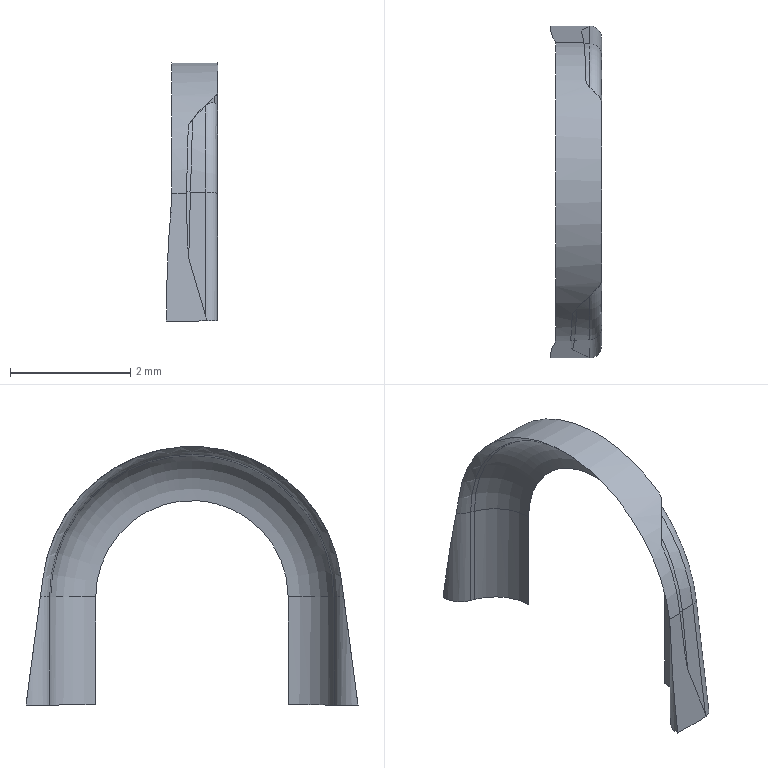Part | STEP file | Basler ace 2 USB3-1-1-1_2 | 1 solid | 37 faces | box 0.85 x 5.522 x 4.3 mm | volume 2.556 mm3 | plane 16 | cylinder 11 | torus 6 | cone 3 | spline 1 | commonest cylinder face diameters 0.4 x4 0.8 x2 1.6 x2 0.3 x1 0.6 x1 5 x1
STEP:
#1=CARTESIAN_POINT('',(-13.565,6.449,-26.303));
#2=VERTEX_POINT('',#1);
#3=CARTESIAN_POINT('',(-13.345,6.67,-26.068));
#4=VERTEX_POINT('',#3);
#5=CARTESIAN_POINT('',(-11.678,8.336,-27.85));
#6=DIRECTION('',(-0.7071,0.7071,0.));
#7=DIRECTION('',(0.7071,0.7071,0.));
#8=AXIS2_PLACEMENT_3D('',#5,#6,#7);
#9=ELLIPSE('',#8,3.451,2.44);
#10=EDGE_CURVE('',#2,#4,#9,.T.);
#11=ORIENTED_EDGE('',*,*,#10,.F.);
#12=CARTESIAN_POINT('',(-13.6,5.933,-27.503));
#13=VERTEX_POINT('',#12);
#14=CARTESIAN_POINT('',(-13.604,7.833,-27.608));
#15=DIRECTION('',(-0.9996,0.000003627,0.02933));
#16=DIRECTION('',(0.02696,0.3938,0.9188));
#17=AXIS2_PLACEMENT_3D('',#14,#15,#16);
#18=ELLIPSE('',#17,2.174,1.873);
#19=EDGE_CURVE('',#13,#2,#18,.T.);
#20=ORIENTED_EDGE('',*,*,#19,.F.);
#21=CARTESIAN_POINT('',(-13.345,5.94,-27.504));
#22=VERTEX_POINT('',#21);
#23=CARTESIAN_POINT('',(-13.345,5.94,-27.504));
#24=DIRECTION('',(-0.9997,-0.02592,0.003643));
#25=VECTOR('',#24,10.);
#26=LINE('',#23,#25);
#27=EDGE_CURVE('',#22,#13,#26,.T.);
#28=ORIENTED_EDGE('',*,*,#27,.F.);
#29=CARTESIAN_POINT('',(-13.345,8.4,-27.85));
#30=DIRECTION('',(1.,0.,0.));
#31=DIRECTION('',(0.,-0.9903,0.1392));
#32=AXIS2_PLACEMENT_3D('',#29,#30,#31);
#33=CIRCLE('',#32,2.484);
#34=EDGE_CURVE('',#4,#22,#33,.T.);
#35=ORIENTED_EDGE('',*,*,#34,.F.);
#36=EDGE_LOOP('',(#11,#20,#28,#35));
#37=FACE_OUTER_BOUND('',#36,.T.);
#38=CARTESIAN_POINT('',(-13.95,8.4,-27.85));
#39=DIRECTION('',(-1.,0.,0.));
#40=DIRECTION('',(0.,-0.9903,-0.1392));
#41=AXIS2_PLACEMENT_3D('',#38,#39,#40);
#42=CONICAL_SURFACE('',#41,2.5,0.02618);
#43=ADVANCED_FACE('',(#37),#42,.T.);
#44=CARTESIAN_POINT('',(-14.,5.639,-29.65));
#45=VERTEX_POINT('',#44);
#46=CARTESIAN_POINT('',(-14.,5.65,-29.65));
#47=VERTEX_POINT('',#46);
#48=CARTESIAN_POINT('',(-14.,5.65,-29.65));
#49=DIRECTION('',(0.,-1.,0.));
#50=VECTOR('',#49,0.011);
#51=LINE('',#48,#50);
#52=EDGE_CURVE('',#45,#47,#51,.F.);
#53=ORIENTED_EDGE('',*,*,#52,.F.);
#54=CARTESIAN_POINT('',(-14.,5.65,-29.567));
#55=VERTEX_POINT('',#54);
#56=CARTESIAN_POINT('',(-14.,5.65,-29.567));
#57=DIRECTION('',(0.,-0.1316,-0.9913));
#58=VECTOR('',#57,0.08356);
#59=LINE('',#56,#58);
#60=EDGE_CURVE('',#55,#45,#59,.T.);
#61=ORIENTED_EDGE('',*,*,#60,.F.);
#62=CARTESIAN_POINT('',(-14.,5.65,-29.65));
#63=DIRECTION('',(0.,0.,1.));
#64=VECTOR('',#63,10.);
#65=LINE('',#62,#64);
#66=EDGE_CURVE('',#47,#55,#65,.T.);
#67=ORIENTED_EDGE('',*,*,#66,.F.);
#68=EDGE_LOOP('',(#53,#61,#67));
#69=FACE_OUTER_BOUND('',#68,.T.);
#70=CARTESIAN_POINT('',(-14.,4.591,-15.027));
#71=DIRECTION('',(1.,0.,0.));
#72=DIRECTION('',(0.,0.,-1.));
#73=AXIS2_PLACEMENT_3D('',#70,#71,#72);
#74=PLANE('',#73);
#75=ADVANCED_FACE('',(#69),#74,.F.);
#76=CARTESIAN_POINT('',(-13.5,5.639,-29.65));
#77=VERTEX_POINT('',#76);
#78=CARTESIAN_POINT('',(-13.5,5.639,-29.65));
#79=DIRECTION('',(-1.,0.,0.));
#80=VECTOR('',#79,0.5);
#81=LINE('',#78,#80);
#82=EDGE_CURVE('',#45,#77,#81,.F.);
#83=ORIENTED_EDGE('',*,*,#82,.F.);
#84=ORIENTED_EDGE('',*,*,#52,.T.);
#85=CARTESIAN_POINT('',(-13.739,6.025,-29.65));
#86=VERTEX_POINT('',#85);
#87=CARTESIAN_POINT('',(-13.6,5.65,-29.65));
#88=DIRECTION('',(0.,0.,-1.));
#89=DIRECTION('',(0.,1.,0.));
#90=AXIS2_PLACEMENT_3D('',#87,#88,#89);
#91=CIRCLE('',#90,0.4);
#92=EDGE_CURVE('',#86,#47,#91,.F.);
#93=ORIENTED_EDGE('',*,*,#92,.F.);
#94=CARTESIAN_POINT('',(-13.672,6.05,-29.65));
#95=VERTEX_POINT('',#94);
#96=CARTESIAN_POINT('',(-13.739,6.025,-29.65));
#97=DIRECTION('',(0.9379,0.3469,0.));
#98=VECTOR('',#97,0.07071);
#99=LINE('',#96,#98);
#100=EDGE_CURVE('',#86,#95,#99,.T.);
#101=ORIENTED_EDGE('',*,*,#100,.T.);
#102=CARTESIAN_POINT('',(-13.5,6.139,-29.65));
#103=VERTEX_POINT('',#102);
#104=CARTESIAN_POINT('',(-13.95,6.8,-29.65));
#105=DIRECTION('',(0.,0.,-1.));
#106=DIRECTION('',(0.,1.,0.));
#107=AXIS2_PLACEMENT_3D('',#104,#105,#106);
#108=CIRCLE('',#107,0.8);
#109=EDGE_CURVE('',#95,#103,#108,.F.);
#110=ORIENTED_EDGE('',*,*,#109,.T.);
#111=CARTESIAN_POINT('',(-13.5,5.639,-29.65));
#112=DIRECTION('',(0.,1.,0.));
#113=VECTOR('',#112,10.);
#114=LINE('',#111,#113);
#115=EDGE_CURVE('',#77,#103,#114,.T.);
#116=ORIENTED_EDGE('',*,*,#115,.F.);
#117=EDGE_LOOP('',(#83,#84,#93,#101,#110,#116));
#118=FACE_OUTER_BOUND('',#117,.T.);
#119=CARTESIAN_POINT('',(-14.2,5.639,-29.65));
#120=DIRECTION('',(0.,0.,-1.));
#121=DIRECTION('',(-1.,0.,0.));
#122=AXIS2_PLACEMENT_3D('',#119,#120,#121);
#123=PLANE('',#122);
#124=ADVANCED_FACE('',(#118),#123,.T.);
#125=CARTESIAN_POINT('',(-13.629,5.777,-28.608));
#126=VERTEX_POINT('',#125);
#127=CARTESIAN_POINT('',(-13.6,5.933,-27.503));
#128=DIRECTION('',(-0.02592,-0.1398,-0.9898));
#129=VECTOR('',#128,10.);
#130=LINE('',#127,#129);
#131=EDGE_CURVE('',#13,#126,#130,.T.);
#132=ORIENTED_EDGE('',*,*,#131,.T.);
#133=CARTESIAN_POINT('',(-13.345,5.648,-29.58));
#134=VERTEX_POINT('',#133);
#135=CARTESIAN_POINT('',(-13.345,5.648,-29.58));
#136=DIRECTION('',(-0.2785,0.1264,0.9521));
#137=VECTOR('',#136,10.);
#138=LINE('',#135,#137);
#139=EDGE_CURVE('',#134,#126,#138,.T.);
#140=ORIENTED_EDGE('',*,*,#139,.F.);
#141=CARTESIAN_POINT('',(-13.345,5.94,-27.504));
#142=DIRECTION('',(0.,-0.1392,-0.9903));
#143=VECTOR('',#142,10.);
#144=LINE('',#141,#143);
#145=EDGE_CURVE('',#22,#134,#144,.T.);
#146=ORIENTED_EDGE('',*,*,#145,.F.);
#147=ORIENTED_EDGE('',*,*,#27,.T.);
#148=EDGE_LOOP('',(#132,#140,#146,#147));
#149=FACE_OUTER_BOUND('',#148,.T.);
#150=CARTESIAN_POINT('',(-13.95,5.621,-29.662));
#151=DIRECTION('',(0.02618,-0.9899,0.1391));
#152=DIRECTION('',(0.,-0.1392,-0.9903));
#153=AXIS2_PLACEMENT_3D('',#150,#151,#152);
#154=PLANE('',#153);
#155=ADVANCED_FACE('',(#149),#154,.T.);
#156=CARTESIAN_POINT('',(-13.667,5.925,-27.5));
#157=VERTEX_POINT('',#156);
#158=CARTESIAN_POINT('',(-13.593,5.636,-27.462));
#159=DIRECTION('',(-0.02592,-0.1398,-0.9898));
#160=DIRECTION('',(-0.02631,0.9899,-0.1391));
#161=AXIS2_PLACEMENT_3D('',#158,#159,#160);
#162=CIRCLE('',#161,0.3004);
#163=EDGE_CURVE('',#157,#13,#162,.T.);
#164=ORIENTED_EDGE('',*,*,#163,.F.);
#165=CARTESIAN_POINT('',(-13.667,5.922,-27.521));
#166=VERTEX_POINT('',#165);
#167=CARTESIAN_POINT('',(-13.652,5.927,-27.513));
#168=DIRECTION('',(-0.2453,0.9608,-0.1293));
#169=DIRECTION('',(0.00731,0.1352,0.9908));
#170=AXIS2_PLACEMENT_3D('',#167,#168,#169);
#171=ELLIPSE('',#170,0.09616,0.01504);
#172=EDGE_CURVE('',#166,#157,#171,.T.);
#173=ORIENTED_EDGE('',*,*,#172,.F.);
#174=CARTESIAN_POINT('',(-13.629,5.777,-28.608));
#175=CARTESIAN_POINT('',(-13.66,5.791,-28.503));
#176=CARTESIAN_POINT('',(-13.667,5.922,-27.521));
#177=(BOUNDED_CURVE()B_SPLINE_CURVE(2,(#174,#175,#176),.UNSPECIFIED.,.F.,.F.)B_SPLINE_CURVE_WITH_KNOTS((3,3),(0.2462,0.3879),.UNSPECIFIED.)CURVE()GEOMETRIC_REPRESENTATION_ITEM()RATIONAL_B_SPLINE_CURVE((0.9685,0.9699,0.9834))REPRESENTATION_ITEM(''));
#178=EDGE_CURVE('',#126,#166,#177,.T.);
#179=ORIENTED_EDGE('',*,*,#178,.F.);
#180=ORIENTED_EDGE('',*,*,#131,.F.);
#181=EDGE_LOOP('',(#164,#173,#179,#180));
#182=FACE_OUTER_BOUND('',#181,.T.);
#183=CARTESIAN_POINT('',(-13.677,5.18,-30.697));
#184=DIRECTION('',(-0.02592,-0.1398,-0.9898));
#185=DIRECTION('',(-0.7173,0.6922,-0.07898));
#186=AXIS2_PLACEMENT_3D('',#183,#184,#185);
#187=CYLINDRICAL_SURFACE('',#186,0.3);
#188=ADVANCED_FACE('',(#182),#187,.F.);
#189=CARTESIAN_POINT('',(-13.637,6.377,-26.381));
#190=VERTEX_POINT('',#189);
#191=CARTESIAN_POINT('',(-13.489,6.525,-25.945));
#192=DIRECTION('',(0.7071,-0.7071,-0.000000002));
#193=DIRECTION('',(-0.4439,-0.4439,-0.7784));
#194=AXIS2_PLACEMENT_3D('',#191,#192,#193);
#195=ELLIPSE('',#194,0.6211,0.1696);
#196=EDGE_CURVE('',#190,#2,#195,.T.);
#197=ORIENTED_EDGE('',*,*,#196,.F.);
#198=CARTESIAN_POINT('',(-13.671,7.831,-27.605));
#199=DIRECTION('',(-0.9996,-0.0009334,0.02666));
#200=DIRECTION('',(0.02413,0.3942,0.9187));
#201=AXIS2_PLACEMENT_3D('',#198,#199,#200);
#202=ELLIPSE('',#201,2.181,1.88);
#203=EDGE_CURVE('',#157,#190,#202,.T.);
#204=ORIENTED_EDGE('',*,*,#203,.F.);
#205=ORIENTED_EDGE('',*,*,#163,.T.);
#206=ORIENTED_EDGE('',*,*,#19,.T.);
#207=EDGE_LOOP('',(#197,#204,#205,#206));
#208=FACE_OUTER_BOUND('',#207,.T.);
#209=CARTESIAN_POINT('',(-13.565,6.449,-26.303));
#210=CARTESIAN_POINT('',(-13.575,6.175,-26.648));
#211=CARTESIAN_POINT('',(-13.588,5.995,-27.067));
#212=CARTESIAN_POINT('',(-13.6,5.933,-27.503));
#213=CARTESIAN_POINT('',(-13.589,6.449,-26.302));
#214=CARTESIAN_POINT('',(-13.599,6.175,-26.647));
#215=CARTESIAN_POINT('',(-13.611,5.995,-27.066));
#216=CARTESIAN_POINT('',(-13.624,5.933,-27.503));
#217=CARTESIAN_POINT('',(-13.612,6.447,-26.299));
#218=CARTESIAN_POINT('',(-13.622,6.172,-26.645));
#219=CARTESIAN_POINT('',(-13.634,5.992,-27.065));
#220=CARTESIAN_POINT('',(-13.647,5.93,-27.502));
#221=CARTESIAN_POINT('',(-13.635,6.442,-26.295));
#222=CARTESIAN_POINT('',(-13.645,6.167,-26.642));
#223=CARTESIAN_POINT('',(-13.657,5.986,-27.062));
#224=CARTESIAN_POINT('',(-13.669,5.924,-27.5));
#225=B_SPLINE_SURFACE_WITH_KNOTS('',3,3,((#209,#210,#211,#212),(#213,#214,#215,#216),(#217,#218,#219,#220),(#221,#222,#223,#224)),.UNSPECIFIED.,.F.,.F.,.F.,(4,4),(4,4),(0.,0.1501),(0.8997,1.43),.UNSPECIFIED.);
#226=ADVANCED_FACE('',(#208),#225,.T.);
#227=CARTESIAN_POINT('',(-13.209,6.806,-25.924));
#228=VERTEX_POINT('',#227);
#229=CARTESIAN_POINT('',(-13.209,6.806,-26.022));
#230=VERTEX_POINT('',#229);
#231=CARTESIAN_POINT('',(-13.209,6.806,-25.924));
#232=DIRECTION('',(0.,0.,-1.));
#233=VECTOR('',#232,10.);
#234=LINE('',#231,#233);
#235=EDGE_CURVE('',#228,#230,#234,.T.);
#236=ORIENTED_EDGE('',*,*,#235,.F.);
#237=CARTESIAN_POINT('',(-11.614,8.4,-27.85));
#238=DIRECTION('',(-0.7071,0.7071,0.));
#239=DIRECTION('',(0.7071,0.7071,0.));
#240=AXIS2_PLACEMENT_3D('',#237,#238,#239);
#241=ELLIPSE('',#240,3.536,2.5);
#242=EDGE_CURVE('',#190,#228,#241,.T.);
#243=ORIENTED_EDGE('',*,*,#242,.F.);
#244=ORIENTED_EDGE('',*,*,#196,.T.);
#245=ORIENTED_EDGE('',*,*,#10,.T.);
#246=CARTESIAN_POINT('',(-13.209,6.806,-26.022));
#247=CARTESIAN_POINT('',(-13.215,6.799,-26.019));
#248=CARTESIAN_POINT('',(-13.223,6.792,-26.017));
#249=CARTESIAN_POINT('',(-13.239,6.775,-26.015));
#250=CARTESIAN_POINT('',(-13.252,6.763,-26.016));
#251=CARTESIAN_POINT('',(-13.29,6.725,-26.025));
#252=CARTESIAN_POINT('',(-13.32,6.694,-26.045));
#253=CARTESIAN_POINT('',(-13.345,6.67,-26.068));
#254=B_SPLINE_CURVE_WITH_KNOTS('',3,(#246,#247,#248,#249,#250,#251,#252,#253),.UNSPECIFIED.,.F.,.F.,(4,2,2,4),(0.1793,0.1821,0.1864,0.1985),.UNSPECIFIED.);
#255=EDGE_CURVE('',#230,#4,#254,.T.);
#256=ORIENTED_EDGE('',*,*,#255,.F.);
#257=EDGE_LOOP('',(#236,#243,#244,#245,#256));
#258=FACE_OUTER_BOUND('',#257,.T.);
#259=CARTESIAN_POINT('',(-13.15,6.864,-25.75));
#260=DIRECTION('',(0.7071,-0.7071,0.));
#261=DIRECTION('',(0.,0.,-1.));
#262=AXIS2_PLACEMENT_3D('',#259,#260,#261);
#263=PLANE('',#262);
#264=ADVANCED_FACE('',(#258),#263,.T.);
#265=CARTESIAN_POINT('',(-13.363,10.148,-26.084));
#266=VERTEX_POINT('',#265);
#267=CARTESIAN_POINT('',(-13.362,10.148,-26.062));
#268=VERTEX_POINT('',#267);
#269=CARTESIAN_POINT('',(-13.363,10.148,-26.084));
#270=DIRECTION('',(0.02617,-0.02617,0.9993));
#271=VECTOR('',#270,10.);
#272=LINE('',#269,#271);
#273=EDGE_CURVE('',#266,#268,#272,.T.);
#274=ORIENTED_EDGE('',*,*,#273,.T.);
#275=CARTESIAN_POINT('',(-13.209,9.994,-25.924));
#276=VERTEX_POINT('',#275);
#277=CARTESIAN_POINT('',(-11.614,8.4,-27.85));
#278=DIRECTION('',(-0.7071,-0.7071,0.));
#279=DIRECTION('',(-0.7071,0.7071,0.));
#280=AXIS2_PLACEMENT_3D('',#277,#278,#279);
#281=ELLIPSE('',#280,3.536,2.5);
#282=EDGE_CURVE('',#276,#268,#281,.T.);
#283=ORIENTED_EDGE('',*,*,#282,.F.);
#284=CARTESIAN_POINT('',(-13.209,9.994,-26.022));
#285=VERTEX_POINT('',#284);
#286=CARTESIAN_POINT('',(-13.209,9.994,-26.022));
#287=DIRECTION('',(0.,0.,1.));
#288=VECTOR('',#287,10.);
#289=LINE('',#286,#288);
#290=EDGE_CURVE('',#285,#276,#289,.T.);
#291=ORIENTED_EDGE('',*,*,#290,.F.);
#292=CARTESIAN_POINT('',(-13.345,10.13,-26.068));
#293=VERTEX_POINT('',#292);
#294=CARTESIAN_POINT('',(-13.345,10.13,-26.068));
#295=CARTESIAN_POINT('',(-13.32,10.106,-26.045));
#296=CARTESIAN_POINT('',(-13.29,10.075,-26.025));
#297=CARTESIAN_POINT('',(-13.252,10.037,-26.016));
#298=CARTESIAN_POINT('',(-13.239,10.025,-26.015));
#299=CARTESIAN_POINT('',(-13.223,10.008,-26.017));
#300=CARTESIAN_POINT('',(-13.215,10.001,-26.019));
#301=CARTESIAN_POINT('',(-13.209,9.994,-26.022));
#302=B_SPLINE_CURVE_WITH_KNOTS('',3,(#294,#295,#296,#297,#298,#299,#300,#301),.UNSPECIFIED.,.F.,.F.,(4,2,2,4),(0.0008828,0.01296,0.01734,0.02009),.UNSPECIFIED.);
#303=EDGE_CURVE('',#293,#285,#302,.T.);
#304=ORIENTED_EDGE('',*,*,#303,.F.);
#305=CARTESIAN_POINT('',(-11.678,8.464,-27.85));
#306=DIRECTION('',(0.7071,0.7071,0.));
#307=DIRECTION('',(-0.7071,0.7071,0.));
#308=AXIS2_PLACEMENT_3D('',#305,#306,#307);
#309=ELLIPSE('',#308,3.451,2.44);
#310=EDGE_CURVE('',#266,#293,#309,.T.);
#311=ORIENTED_EDGE('',*,*,#310,.F.);
#312=EDGE_LOOP('',(#274,#283,#291,#304,#311));
#313=FACE_OUTER_BOUND('',#312,.T.);
#314=CARTESIAN_POINT('',(-14.05,10.836,-25.75));
#315=DIRECTION('',(0.7071,0.7071,0.));
#316=DIRECTION('',(0.,0.,-1.));
#317=AXIS2_PLACEMENT_3D('',#314,#315,#316);
#318=PLANE('',#317);
#319=ADVANCED_FACE('',(#313),#318,.T.);
#320=CARTESIAN_POINT('',(-13.41,10.257,-26.198));
#321=VERTEX_POINT('',#320);
#322=CARTESIAN_POINT('',(-13.41,10.257,-26.198));
#323=CARTESIAN_POINT('',(-13.409,10.24,-26.179));
#324=CARTESIAN_POINT('',(-13.406,10.222,-26.159));
#325=CARTESIAN_POINT('',(-13.391,10.185,-26.12));
#326=CARTESIAN_POINT('',(-13.38,10.166,-26.101));
#327=CARTESIAN_POINT('',(-13.364,10.15,-26.086));
#328=CARTESIAN_POINT('',(-13.363,10.149,-26.085));
#329=CARTESIAN_POINT('',(-13.363,10.148,-26.084));
#330=B_SPLINE_CURVE_WITH_KNOTS('',3,(#322,#323,#324,#325,#326,#327,#328,#329),.UNSPECIFIED.,.F.,.F.,(4,2,2,4),(-0.02801,-0.02048,-0.0125,-0.01215),.UNSPECIFIED.);
#331=EDGE_CURVE('',#321,#266,#330,.T.);
#332=ORIENTED_EDGE('',*,*,#331,.F.);
#333=CARTESIAN_POINT('',(-13.409,10.257,-26.176));
#334=VERTEX_POINT('',#333);
#335=CARTESIAN_POINT('',(-13.409,10.257,-26.176));
#336=DIRECTION('',(-0.02617,0.02617,-0.9993));
#337=VECTOR('',#336,10.);
#338=LINE('',#335,#337);
#339=EDGE_CURVE('',#321,#334,#338,.F.);
#340=ORIENTED_EDGE('',*,*,#339,.T.);
#341=CARTESIAN_POINT('',(-13.362,10.148,-26.062));
#342=CARTESIAN_POINT('',(-13.377,10.163,-26.077));
#343=CARTESIAN_POINT('',(-13.389,10.181,-26.096));
#344=CARTESIAN_POINT('',(-13.405,10.219,-26.135));
#345=CARTESIAN_POINT('',(-13.408,10.239,-26.156));
#346=CARTESIAN_POINT('',(-13.409,10.257,-26.176));
#347=CARTESIAN_POINT('',(-13.409,10.257,-26.176));
#348=CARTESIAN_POINT('',(-13.409,10.257,-26.176));
#349=B_SPLINE_CURVE_WITH_KNOTS('',3,(#341,#342,#343,#344,#345,#346,#347,#348),.UNSPECIFIED.,.F.,.F.,(4,2,2,4),(0.01252,0.02045,0.02838,0.0284),.UNSPECIFIED.);
#350=EDGE_CURVE('',#268,#334,#349,.T.);
#351=ORIENTED_EDGE('',*,*,#350,.F.);
#352=ORIENTED_EDGE('',*,*,#273,.F.);
#353=EDGE_LOOP('',(#332,#340,#351,#352));
#354=FACE_OUTER_BOUND('',#353,.T.);
#355=CARTESIAN_POINT('',(-13.299,10.296,-27.695));
#356=DIRECTION('',(0.02617,-0.02617,0.9993));
#357=DIRECTION('',(-0.9238,-0.3827,0.01417));
#358=AXIS2_PLACEMENT_3D('',#355,#356,#357);
#359=CYLINDRICAL_SURFACE('',#358,0.15);
#360=ADVANCED_FACE('',(#354),#359,.F.);
#361=CARTESIAN_POINT('',(-13.444,10.863,-27.504));
#362=VERTEX_POINT('',#361);
#363=CARTESIAN_POINT('',(-13.453,8.4,-27.852));
#364=DIRECTION('',(0.9997,0.,-0.02618));
#365=DIRECTION('',(0.02618,0.,0.9997));
#366=AXIS2_PLACEMENT_3D('',#363,#364,#365);
#367=ELLIPSE('',#366,2.488,2.487);
#368=EDGE_CURVE('',#362,#321,#367,.T.);
#369=ORIENTED_EDGE('',*,*,#368,.T.);
#370=ORIENTED_EDGE('',*,*,#331,.T.);
#371=ORIENTED_EDGE('',*,*,#310,.T.);
#372=CARTESIAN_POINT('',(-13.345,10.86,-27.504));
#373=VERTEX_POINT('',#372);
#374=CARTESIAN_POINT('',(-13.345,8.4,-27.85));
#375=DIRECTION('',(1.,0.,0.));
#376=DIRECTION('',(0.,0.6965,0.7175));
#377=AXIS2_PLACEMENT_3D('',#374,#375,#376);
#378=CIRCLE('',#377,2.484);
#379=EDGE_CURVE('',#373,#293,#378,.T.);
#380=ORIENTED_EDGE('',*,*,#379,.F.);
#381=CARTESIAN_POINT('',(-13.444,10.863,-27.504));
#382=DIRECTION('',(0.9997,-0.02592,-0.003643));
#383=VECTOR('',#382,10.);
#384=LINE('',#381,#383);
#385=EDGE_CURVE('',#362,#373,#384,.T.);
#386=ORIENTED_EDGE('',*,*,#385,.F.);
#387=EDGE_LOOP('',(#369,#370,#371,#380,#386));
#388=FACE_OUTER_BOUND('',#387,.T.);
#389=CARTESIAN_POINT('',(-13.95,8.4,-27.85));
#390=DIRECTION('',(-1.,0.,0.));
#391=DIRECTION('',(0.,-0.9903,-0.1392));
#392=AXIS2_PLACEMENT_3D('',#389,#390,#391);
#393=CONICAL_SURFACE('',#392,2.5,0.02618);
#394=ADVANCED_FACE('',(#388),#393,.T.);
#395=ORIENTED_EDGE('',*,*,#379,.T.);
#396=ORIENTED_EDGE('',*,*,#303,.T.);
#397=CARTESIAN_POINT('',(-13.15,9.853,-26.087));
#398=VERTEX_POINT('',#397);
#399=CARTESIAN_POINT('',(-13.15,9.853,-26.087));
#400=CARTESIAN_POINT('',(-13.15,9.853,-26.087));
#401=CARTESIAN_POINT('',(-13.15,9.854,-26.087));
#402=CARTESIAN_POINT('',(-13.15,9.87,-26.079));
#403=CARTESIAN_POINT('',(-13.152,9.885,-26.072));
#404=CARTESIAN_POINT('',(-13.159,9.915,-26.058));
#405=CARTESIAN_POINT('',(-13.164,9.929,-26.052));
#406=CARTESIAN_POINT('',(-13.181,9.961,-26.037));
#407=CARTESIAN_POINT('',(-13.193,9.979,-26.029));
#408=CARTESIAN_POINT('',(-13.209,9.994,-26.022));
#409=B_SPLINE_CURVE_WITH_KNOTS('',3,(#399,#400,#401,#402,#403,#404,#405,#406,#407,#408),.UNSPECIFIED.,.F.,.F.,(4,2,2,2,4),(-0.0002215,0.,0.005038,0.01002,0.01684),.UNSPECIFIED.);
#410=EDGE_CURVE('',#398,#285,#409,.T.);
#411=ORIENTED_EDGE('',*,*,#410,.F.);
#412=CARTESIAN_POINT('',(-13.15,10.662,-27.532));
#413=VERTEX_POINT('',#412);
#414=CARTESIAN_POINT('',(-13.15,10.662,-27.532));
#415=CARTESIAN_POINT('',(-13.15,10.653,-27.47));
#416=CARTESIAN_POINT('',(-13.15,10.642,-27.409));
#417=CARTESIAN_POINT('',(-13.15,10.615,-27.288));
#418=CARTESIAN_POINT('',(-13.15,10.599,-27.228));
#419=CARTESIAN_POINT('',(-13.15,10.562,-27.11));
#420=CARTESIAN_POINT('',(-13.15,10.541,-27.051));
#421=CARTESIAN_POINT('',(-13.15,10.494,-26.936));
#422=CARTESIAN_POINT('',(-13.15,10.469,-26.88));
#423=CARTESIAN_POINT('',(-13.15,10.426,-26.794));
#424=CARTESIAN_POINT('',(-13.15,10.41,-26.764));
#425=CARTESIAN_POINT('',(-13.15,10.363,-26.68));
#426=CARTESIAN_POINT('',(-13.15,10.33,-26.627));
#427=CARTESIAN_POINT('',(-13.15,10.262,-26.525));
#428=CARTESIAN_POINT('',(-13.15,10.225,-26.475));
#429=CARTESIAN_POINT('',(-13.15,10.148,-26.379));
#430=CARTESIAN_POINT('',(-13.15,10.108,-26.332));
#431=CARTESIAN_POINT('',(-13.15,10.024,-26.242));
#432=CARTESIAN_POINT('',(-13.15,9.98,-26.199));
#433=CARTESIAN_POINT('',(-13.15,9.908,-26.134));
#434=CARTESIAN_POINT('',(-13.15,9.881,-26.11));
#435=CARTESIAN_POINT('',(-13.15,9.853,-26.087));
#436=B_SPLINE_CURVE_WITH_KNOTS('',3,(#414,#415,#416,#417,#418,#419,#420,#421,#422,#423,#424,#425,#426,#427,#428,#429,#430,#431,#432,#433,#434,#435),.UNSPECIFIED.,.F.,.F.,(4,2,2,2,2,2,2,2,2,2,4),(0.,0.1091,0.2198,0.3303,0.4398,0.5,0.6084,0.7183,0.8282,0.9369,1.),.UNSPECIFIED.);
#437=EDGE_CURVE('',#413,#398,#436,.T.);
#438=ORIENTED_EDGE('',*,*,#437,.F.);
#439=CARTESIAN_POINT('',(-13.35,10.662,-27.532));
#440=DIRECTION('',(0.,0.1392,-0.9903));
#441=DIRECTION('',(1.,0.,0.));
#442=AXIS2_PLACEMENT_3D('',#439,#440,#441);
#443=CIRCLE('',#442,0.2);
#444=EDGE_CURVE('',#373,#413,#443,.T.);
#445=ORIENTED_EDGE('',*,*,#444,.F.);
#446=EDGE_LOOP('',(#395,#396,#411,#438,#445));
#447=FACE_OUTER_BOUND('',#446,.T.);
#448=CARTESIAN_POINT('',(-13.35,8.4,-27.85));
#449=DIRECTION('',(-1.,0.,0.));
#450=DIRECTION('',(0.,0.,1.));
#451=AXIS2_PLACEMENT_3D('',#448,#449,#450);
#452=TOROIDAL_SURFACE('',#451,2.284,0.2);
#453=ADVANCED_FACE('',(#447),#452,.T.);
#454=ORIENTED_EDGE('',*,*,#290,.T.);
#455=CARTESIAN_POINT('',(-13.184,9.964,-25.9));
#456=VERTEX_POINT('',#455);
#457=CARTESIAN_POINT('',(-13.184,9.964,-25.9));
#458=CARTESIAN_POINT('',(-13.191,9.975,-25.909));
#459=CARTESIAN_POINT('',(-13.2,9.985,-25.917));
#460=CARTESIAN_POINT('',(-13.209,9.994,-25.924));
#461=B_SPLINE_CURVE_WITH_KNOTS('',3,(#457,#458,#459,#460),.UNSPECIFIED.,.F.,.F.,(4,4),(-0.02057,-0.01615),.UNSPECIFIED.);
#462=EDGE_CURVE('',#456,#276,#461,.T.);
#463=ORIENTED_EDGE('',*,*,#462,.F.);
#464=CARTESIAN_POINT('',(-13.15,9.853,-25.9));
#465=VERTEX_POINT('',#464);
#466=CARTESIAN_POINT('',(-13.35,9.853,-25.9));
#467=DIRECTION('',(0.,0.,-1.));
#468=DIRECTION('',(1.,0.,0.));
#469=AXIS2_PLACEMENT_3D('',#466,#467,#468);
#470=CIRCLE('',#469,0.2);
#471=EDGE_CURVE('',#456,#465,#470,.T.);
#472=ORIENTED_EDGE('',*,*,#471,.T.);
#473=CARTESIAN_POINT('',(-13.15,9.853,-26.087));
#474=DIRECTION('',(0.,0.,1.));
#475=VECTOR('',#474,10.);
#476=LINE('',#473,#475);
#477=EDGE_CURVE('',#398,#465,#476,.T.);
#478=ORIENTED_EDGE('',*,*,#477,.F.);
#479=ORIENTED_EDGE('',*,*,#410,.T.);
#480=EDGE_LOOP('',(#454,#463,#472,#478,#479));
#481=FACE_OUTER_BOUND('',#480,.T.);
#482=CARTESIAN_POINT('',(-13.35,9.853,-26.628));
#483=DIRECTION('',(0.,0.,-1.));
#484=DIRECTION('',(0.9239,0.3827,0.));
#485=AXIS2_PLACEMENT_3D('',#482,#483,#484);
#486=CYLINDRICAL_SURFACE('',#485,0.2);
#487=ADVANCED_FACE('',(#481),#486,.T.);
#488=ORIENTED_EDGE('',*,*,#471,.F.);
#489=CARTESIAN_POINT('',(-13.15,9.906,-25.855));
#490=VERTEX_POINT('',#489);
#491=CARTESIAN_POINT('',(-13.15,9.906,-25.855));
#492=CARTESIAN_POINT('',(-13.152,9.91,-25.857));
#493=CARTESIAN_POINT('',(-13.154,9.914,-25.86));
#494=CARTESIAN_POINT('',(-13.156,9.917,-25.863));
#495=CARTESIAN_POINT('',(-13.164,9.932,-25.875));
#496=CARTESIAN_POINT('',(-13.172,9.947,-25.886));
#497=CARTESIAN_POINT('',(-13.182,9.961,-25.897));
#498=CARTESIAN_POINT('',(-13.183,9.962,-25.898));
#499=CARTESIAN_POINT('',(-13.183,9.963,-25.899));
#500=CARTESIAN_POINT('',(-13.184,9.964,-25.9));
#501=B_SPLINE_CURVE_WITH_KNOTS('',3,(#491,#492,#493,#494,#495,#496,#497,#498,#499,#500),.UNSPECIFIED.,.F.,.F.,(4,3,3,4),(0.06206,0.06324,0.06798,0.06839),.UNSPECIFIED.);
#502=EDGE_CURVE('',#490,#456,#501,.T.);
#503=ORIENTED_EDGE('',*,*,#502,.F.);
#504=CARTESIAN_POINT('',(-13.15,9.853,-25.9));
#505=CARTESIAN_POINT('',(-13.15,9.862,-25.892));
#506=CARTESIAN_POINT('',(-13.15,9.871,-25.884));
#507=CARTESIAN_POINT('',(-13.15,9.881,-25.876));
#508=CARTESIAN_POINT('',(-13.15,9.889,-25.869));
#509=CARTESIAN_POINT('',(-13.15,9.898,-25.862));
#510=CARTESIAN_POINT('',(-13.15,9.906,-25.855));
#511=B_SPLINE_CURVE_WITH_KNOTS('',3,(#504,#505,#506,#507,#508,#509,#510),.UNSPECIFIED.,.F.,.F.,(4,3,4),(0.,0.003624,0.006665),.UNSPECIFIED.);
#512=EDGE_CURVE('',#465,#490,#511,.T.);
#513=ORIENTED_EDGE('',*,*,#512,.F.);
#514=EDGE_LOOP('',(#488,#503,#513));
#515=FACE_OUTER_BOUND('',#514,.T.);
#516=CARTESIAN_POINT('',(-13.35,9.853,-25.9));
#517=DIRECTION('',(0.,0.,1.));
#518=DIRECTION('',(1.,0.,0.));
#519=AXIS2_PLACEMENT_3D('',#516,#517,#518);
#520=TOROIDAL_SURFACE('',#519,0.35,0.15);
#521=ADVANCED_FACE('',(#515),#520,.F.);
#522=CARTESIAN_POINT('',(-13.15,6.894,-25.855));
#523=VERTEX_POINT('',#522);
#524=CARTESIAN_POINT('',(-13.15,6.947,-25.9));
#525=VERTEX_POINT('',#524);
#526=CARTESIAN_POINT('',(-13.15,6.894,-25.855));
#527=CARTESIAN_POINT('',(-13.15,6.906,-25.864));
#528=CARTESIAN_POINT('',(-13.15,6.917,-25.874));
#529=CARTESIAN_POINT('',(-13.15,6.928,-25.884));
#530=CARTESIAN_POINT('',(-13.15,6.935,-25.889));
#531=CARTESIAN_POINT('',(-13.15,6.941,-25.895));
#532=CARTESIAN_POINT('',(-13.15,6.947,-25.9));
#533=B_SPLINE_CURVE_WITH_KNOTS('',3,(#526,#527,#528,#529,#530,#531,#532),.UNSPECIFIED.,.F.,.F.,(4,3,4),(0.1036,0.1078,0.1102),.UNSPECIFIED.);
#534=EDGE_CURVE('',#523,#525,#533,.T.);
#535=ORIENTED_EDGE('',*,*,#534,.F.);
#536=CARTESIAN_POINT('',(-13.184,6.836,-25.9));
#537=VERTEX_POINT('',#536);
#538=CARTESIAN_POINT('',(-13.184,6.836,-25.9));
#539=CARTESIAN_POINT('',(-13.17,6.856,-25.884));
#540=CARTESIAN_POINT('',(-13.16,6.875,-25.869));
#541=CARTESIAN_POINT('',(-13.15,6.894,-25.855));
#542=B_SPLINE_CURVE_WITH_KNOTS('',3,(#538,#539,#540,#541),.UNSPECIFIED.,.F.,.F.,(4,4),(0.08375,0.09033),.UNSPECIFIED.);
#543=EDGE_CURVE('',#537,#523,#542,.T.);
#544=ORIENTED_EDGE('',*,*,#543,.F.);
#545=CARTESIAN_POINT('',(-13.35,6.947,-25.9));
#546=DIRECTION('',(0.,0.,-1.));
#547=DIRECTION('',(0.8293,-0.5589,0.));
#548=AXIS2_PLACEMENT_3D('',#545,#546,#547);
#549=CIRCLE('',#548,0.2);
#550=EDGE_CURVE('',#525,#537,#549,.T.);
#551=ORIENTED_EDGE('',*,*,#550,.F.);
#552=EDGE_LOOP('',(#535,#544,#551));
#553=FACE_OUTER_BOUND('',#552,.T.);
#554=CARTESIAN_POINT('',(-13.35,6.947,-25.9));
#555=DIRECTION('',(0.,0.,1.));
#556=DIRECTION('',(1.,0.,0.));
#557=AXIS2_PLACEMENT_3D('',#554,#555,#556);
#558=TOROIDAL_SURFACE('',#557,0.35,0.15);
#559=ADVANCED_FACE('',(#553),#558,.F.);
#560=ORIENTED_EDGE('',*,*,#550,.T.);
#561=CARTESIAN_POINT('',(-13.32,6.927,-25.842));
#562=DIRECTION('',(-0.06324,-0.5986,0.7985));
#563=DIRECTION('',(-0.2251,-0.7709,-0.5958));
#564=AXIS2_PLACEMENT_3D('',#561,#562,#563);
#565=ELLIPSE('',#564,0.2235,0.1667);
#566=EDGE_CURVE('',#228,#537,#565,.T.);
#567=ORIENTED_EDGE('',*,*,#566,.F.);
#568=ORIENTED_EDGE('',*,*,#235,.T.);
#569=CARTESIAN_POINT('',(-13.15,6.947,-26.087));
#570=VERTEX_POINT('',#569);
#571=CARTESIAN_POINT('',(-13.15,6.947,-26.087));
#572=CARTESIAN_POINT('',(-13.15,6.947,-26.087));
#573=CARTESIAN_POINT('',(-13.15,6.946,-26.087));
#574=CARTESIAN_POINT('',(-13.15,6.93,-26.079));
#575=CARTESIAN_POINT('',(-13.152,6.915,-26.072));
#576=CARTESIAN_POINT('',(-13.159,6.885,-26.058));
#577=CARTESIAN_POINT('',(-13.164,6.871,-26.052));
#578=CARTESIAN_POINT('',(-13.181,6.839,-26.037));
#579=CARTESIAN_POINT('',(-13.193,6.821,-26.029));
#580=CARTESIAN_POINT('',(-13.209,6.806,-26.022));
#581=B_SPLINE_CURVE_WITH_KNOTS('',3,(#571,#572,#573,#574,#575,#576,#577,#578,#579,#580),.UNSPECIFIED.,.F.,.F.,(4,2,2,2,4),(-0.0661,-0.06588,-0.06084,-0.05585,-0.04904),.UNSPECIFIED.);
#582=EDGE_CURVE('',#570,#230,#581,.T.);
#583=ORIENTED_EDGE('',*,*,#582,.F.);
#584=CARTESIAN_POINT('',(-13.15,6.947,-25.9));
#585=DIRECTION('',(0.,0.,-1.));
#586=VECTOR('',#585,10.);
#587=LINE('',#584,#586);
#588=EDGE_CURVE('',#525,#570,#587,.T.);
#589=ORIENTED_EDGE('',*,*,#588,.F.);
#590=EDGE_LOOP('',(#560,#567,#568,#583,#589));
#591=FACE_OUTER_BOUND('',#590,.T.);
#592=CARTESIAN_POINT('',(-13.35,6.947,-26.628));
#593=DIRECTION('',(0.,0.,1.));
#594=DIRECTION('',(0.9239,-0.3827,0.));
#595=AXIS2_PLACEMENT_3D('',#592,#593,#594);
#596=CYLINDRICAL_SURFACE('',#595,0.2);
#597=ADVANCED_FACE('',(#591),#596,.T.);
#598=CARTESIAN_POINT('',(-13.15,6.138,-27.532));
#599=VERTEX_POINT('',#598);
#600=CARTESIAN_POINT('',(-13.15,6.947,-26.087));
#601=CARTESIAN_POINT('',(-13.15,6.899,-26.127));
#602=CARTESIAN_POINT('',(-13.15,6.853,-26.168));
#603=CARTESIAN_POINT('',(-13.15,6.764,-26.255));
#604=CARTESIAN_POINT('',(-13.15,6.721,-26.3));
#605=CARTESIAN_POINT('',(-13.15,6.639,-26.393));
#606=CARTESIAN_POINT('',(-13.15,6.601,-26.442));
#607=CARTESIAN_POINT('',(-13.15,6.527,-26.541));
#608=CARTESIAN_POINT('',(-13.15,6.492,-26.592));
#609=CARTESIAN_POINT('',(-13.15,6.441,-26.674));
#610=CARTESIAN_POINT('',(-13.15,6.424,-26.704));
#611=CARTESIAN_POINT('',(-13.15,6.377,-26.788));
#612=CARTESIAN_POINT('',(-13.15,6.349,-26.843));
#613=CARTESIAN_POINT('',(-13.15,6.298,-26.955));
#614=CARTESIAN_POINT('',(-13.15,6.274,-27.012));
#615=CARTESIAN_POINT('',(-13.15,6.232,-27.128));
#616=CARTESIAN_POINT('',(-13.15,6.213,-27.187));
#617=CARTESIAN_POINT('',(-13.15,6.181,-27.305));
#618=CARTESIAN_POINT('',(-13.15,6.167,-27.365));
#619=CARTESIAN_POINT('',(-13.15,6.149,-27.461));
#620=CARTESIAN_POINT('',(-13.15,6.143,-27.496));
#621=CARTESIAN_POINT('',(-13.15,6.138,-27.532));
#622=B_SPLINE_CURVE_WITH_KNOTS('',3,(#600,#601,#602,#603,#604,#605,#606,#607,#608,#609,#610,#611,#612,#613,#614,#615,#616,#617,#618,#619,#620,#621),.UNSPECIFIED.,.F.,.F.,(4,2,2,2,2,2,2,2,2,2,4),(0.,0.1091,0.2198,0.3303,0.4398,0.5,0.6084,0.7183,0.8282,0.9369,1.),.UNSPECIFIED.);
#623=EDGE_CURVE('',#570,#599,#622,.T.);
#624=ORIENTED_EDGE('',*,*,#623,.F.);
#625=ORIENTED_EDGE('',*,*,#582,.T.);
#626=ORIENTED_EDGE('',*,*,#255,.T.);
#627=ORIENTED_EDGE('',*,*,#34,.T.);
#628=CARTESIAN_POINT('',(-13.35,6.138,-27.532));
#629=DIRECTION('',(0.,-0.1392,-0.9903));
#630=DIRECTION('',(0.02618,-0.9899,0.1391));
#631=AXIS2_PLACEMENT_3D('',#628,#629,#630);
#632=CIRCLE('',#631,0.2);
#633=EDGE_CURVE('',#599,#22,#632,.T.);
#634=ORIENTED_EDGE('',*,*,#633,.F.);
#635=EDGE_LOOP('',(#624,#625,#626,#627,#634));
#636=FACE_OUTER_BOUND('',#635,.T.);
#637=CARTESIAN_POINT('',(-13.35,8.4,-27.85));
#638=DIRECTION('',(-1.,0.,0.));
#639=DIRECTION('',(0.,0.,1.));
#640=AXIS2_PLACEMENT_3D('',#637,#638,#639);
#641=TOROIDAL_SURFACE('',#640,2.284,0.2);
#642=ADVANCED_FACE('',(#636),#641,.T.);
#643=ORIENTED_EDGE('',*,*,#145,.T.);
#644=CARTESIAN_POINT('',(-13.335,5.64,-29.646));
#645=VERTEX_POINT('',#644);
#646=CARTESIAN_POINT('',(-13.335,5.64,-29.646));
#647=CARTESIAN_POINT('',(-13.34,5.646,-29.597));
#648=CARTESIAN_POINT('',(-13.345,5.648,-29.58));
#649=(BOUNDED_CURVE()B_SPLINE_CURVE(2,(#646,#647,#648),.UNSPECIFIED.,.F.,.F.)B_SPLINE_CURVE_WITH_KNOTS((3,3),(-0.1508,-0.1314),.UNSPECIFIED.)CURVE()GEOMETRIC_REPRESENTATION_ITEM()RATIONAL_B_SPLINE_CURVE((0.9784,0.9775,0.9772))REPRESENTATION_ITEM(''));
#650=EDGE_CURVE('',#645,#134,#649,.T.);
#651=ORIENTED_EDGE('',*,*,#650,.F.);
#652=CARTESIAN_POINT('',(-13.15,5.842,-29.641));
#653=VERTEX_POINT('',#652);
#654=CARTESIAN_POINT('',(-13.35,5.841,-29.646));
#655=DIRECTION('',(0.02618,0.,-0.9997));
#656=DIRECTION('',(-0.183,-0.9831,-0.004793));
#657=AXIS2_PLACEMENT_3D('',#654,#655,#656);
#658=ELLIPSE('',#657,0.202,0.2);
#659=EDGE_CURVE('',#653,#645,#658,.T.);
#660=ORIENTED_EDGE('',*,*,#659,.F.);
#661=CARTESIAN_POINT('',(-13.15,6.138,-27.532));
#662=DIRECTION('',(0.,-0.1392,-0.9903));
#663=VECTOR('',#662,10.);
#664=LINE('',#661,#663);
#665=EDGE_CURVE('',#599,#653,#664,.T.);
#666=ORIENTED_EDGE('',*,*,#665,.F.);
#667=ORIENTED_EDGE('',*,*,#633,.T.);
#668=EDGE_LOOP('',(#643,#651,#660,#666,#667));
#669=FACE_OUTER_BOUND('',#668,.T.);
#670=CARTESIAN_POINT('',(-13.35,5.921,-29.074));
#671=DIRECTION('',(0.,0.1392,0.9903));
#672=DIRECTION('',(0.7163,-0.691,0.09711));
#673=AXIS2_PLACEMENT_3D('',#670,#671,#672);
#674=CYLINDRICAL_SURFACE('',#673,0.2);
#675=ADVANCED_FACE('',(#669),#674,.T.);
#676=CARTESIAN_POINT('',(-13.5,5.639,-29.65));
#677=DIRECTION('',(0.9997,0.003476,0.02618));
#678=VECTOR('',#677,0.1651);
#679=LINE('',#676,#678);
#680=EDGE_CURVE('',#77,#645,#679,.T.);
#681=ORIENTED_EDGE('',*,*,#680,.F.);
#682=ORIENTED_EDGE('',*,*,#115,.T.);
#683=CARTESIAN_POINT('',(-13.15,6.8,-29.641));
#684=VERTEX_POINT('',#683);
#685=CARTESIAN_POINT('',(-13.95,6.8,-29.662));
#686=DIRECTION('',(-0.02618,-0.000000012,0.9997));
#687=DIRECTION('',(0.9914,0.1285,0.02596));
#688=AXIS2_PLACEMENT_3D('',#685,#686,#687);
#689=ELLIPSE('',#688,0.8002,0.7999);
#690=EDGE_CURVE('',#103,#684,#689,.T.);
#691=ORIENTED_EDGE('',*,*,#690,.T.);
#692=CARTESIAN_POINT('',(-13.15,5.842,-29.641));
#693=DIRECTION('',(0.,1.,0.));
#694=VECTOR('',#693,0.9584);
#695=LINE('',#692,#694);
#696=EDGE_CURVE('',#653,#684,#695,.T.);
#697=ORIENTED_EDGE('',*,*,#696,.F.);
#698=ORIENTED_EDGE('',*,*,#659,.T.);
#699=EDGE_LOOP('',(#681,#682,#691,#697,#698));
#700=FACE_OUTER_BOUND('',#699,.T.);
#701=CARTESIAN_POINT('',(-13.95,11.179,-29.662));
#702=DIRECTION('',(0.02618,0.,-0.9997));
#703=DIRECTION('',(-0.9997,0.,-0.02618));
#704=AXIS2_PLACEMENT_3D('',#701,#702,#703);
#705=PLANE('',#704);
#706=ADVANCED_FACE('',(#700),#705,.T.);
#707=CARTESIAN_POINT('',(-13.672,6.05,-27.85));
#708=VERTEX_POINT('',#707);
#709=CARTESIAN_POINT('',(-13.672,6.05,-27.85));
#710=DIRECTION('',(0.,0.,-1.));
#711=VECTOR('',#710,10.);
#712=LINE('',#709,#711);
#713=EDGE_CURVE('',#95,#708,#712,.F.);
#714=ORIENTED_EDGE('',*,*,#713,.T.);
#715=CARTESIAN_POINT('',(-13.15,6.8,-27.85));
#716=VERTEX_POINT('',#715);
#717=CARTESIAN_POINT('',(-13.95,6.8,-27.85));
#718=DIRECTION('',(0.,0.,-1.));
#719=DIRECTION('',(0.3469,-0.9379,0.));
#720=AXIS2_PLACEMENT_3D('',#717,#718,#719);
#721=CIRCLE('',#720,0.8);
#722=EDGE_CURVE('',#708,#716,#721,.F.);
#723=ORIENTED_EDGE('',*,*,#722,.T.);
#724=CARTESIAN_POINT('',(-13.15,6.8,-29.641));
#725=DIRECTION('',(0.,0.,1.));
#726=VECTOR('',#725,10.);
#727=LINE('',#724,#726);
#728=EDGE_CURVE('',#684,#716,#727,.T.);
#729=ORIENTED_EDGE('',*,*,#728,.F.);
#730=ORIENTED_EDGE('',*,*,#690,.F.);
#731=ORIENTED_EDGE('',*,*,#109,.F.);
#732=EDGE_LOOP('',(#714,#723,#729,#730,#731));
#733=FACE_OUTER_BOUND('',#732,.T.);
#734=CARTESIAN_POINT('',(-13.95,6.8,-27.85));
#735=DIRECTION('',(0.,0.,-1.));
#736=DIRECTION('',(0.3469,-0.9379,0.));
#737=AXIS2_PLACEMENT_3D('',#734,#735,#736);
#738=CYLINDRICAL_SURFACE('',#737,0.8);
#739=ADVANCED_FACE('',(#733),#738,.F.);
#740=ORIENTED_EDGE('',*,*,#100,.F.);
#741=CARTESIAN_POINT('',(-13.739,6.025,-27.85));
#742=VERTEX_POINT('',#741);
#743=CARTESIAN_POINT('',(-13.739,6.025,-27.85));
#744=DIRECTION('',(0.,0.,-1.));
#745=VECTOR('',#744,10.);
#746=LINE('',#743,#745);
#747=EDGE_CURVE('',#742,#86,#746,.T.);
#748=ORIENTED_EDGE('',*,*,#747,.F.);
#749=CARTESIAN_POINT('',(-13.672,6.05,-27.85));
#750=DIRECTION('',(-0.9379,-0.3469,0.));
#751=VECTOR('',#750,10.);
#752=LINE('',#749,#751);
#753=EDGE_CURVE('',#742,#708,#752,.F.);
#754=ORIENTED_EDGE('',*,*,#753,.T.);
#755=ORIENTED_EDGE('',*,*,#713,.F.);
#756=EDGE_LOOP('',(#740,#748,#754,#755));
#757=FACE_OUTER_BOUND('',#756,.T.);
#758=CARTESIAN_POINT('',(-13.672,6.05,-27.85));
#759=DIRECTION('',(0.3469,-0.9379,0.));
#760=DIRECTION('',(0.,0.,-1.));
#761=AXIS2_PLACEMENT_3D('',#758,#759,#760);
#762=PLANE('',#761);
#763=ADVANCED_FACE('',(#757),#762,.F.);
#764=ORIENTED_EDGE('',*,*,#66,.T.);
#765=CARTESIAN_POINT('',(-13.929,5.878,-27.85));
#766=VERTEX_POINT('',#765);
#767=CARTESIAN_POINT('',(-13.6,5.65,-29.567));
#768=DIRECTION('',(0.,-0.9913,0.1316));
#769=DIRECTION('',(0.,-0.1316,-0.9913));
#770=AXIS2_PLACEMENT_3D('',#767,#768,#769);
#771=ELLIPSE('',#770,3.038,0.4);
#772=EDGE_CURVE('',#766,#55,#771,.T.);
#773=ORIENTED_EDGE('',*,*,#772,.F.);
#774=CARTESIAN_POINT('',(-13.6,5.65,-27.85));
#775=DIRECTION('',(0.,0.,1.));
#776=DIRECTION('',(-0.8216,0.5701,0.));
#777=AXIS2_PLACEMENT_3D('',#774,#775,#776);
#778=CIRCLE('',#777,0.4);
#779=EDGE_CURVE('',#742,#766,#778,.T.);
#780=ORIENTED_EDGE('',*,*,#779,.F.);
#781=ORIENTED_EDGE('',*,*,#747,.T.);
#782=ORIENTED_EDGE('',*,*,#92,.T.);
#783=EDGE_LOOP('',(#764,#773,#780,#781,#782));
#784=FACE_OUTER_BOUND('',#783,.T.);
#785=CARTESIAN_POINT('',(-13.6,5.65,-27.85));
#786=DIRECTION('',(0.,0.,-1.));
#787=DIRECTION('',(0.3469,-0.9379,0.));
#788=AXIS2_PLACEMENT_3D('',#785,#786,#787);
#789=CYLINDRICAL_SURFACE('',#788,0.4);
#790=ADVANCED_FACE('',(#784),#789,.T.);
#791=CARTESIAN_POINT('',(-13.912,5.922,-27.521));
#792=VERTEX_POINT('',#791);
#793=CARTESIAN_POINT('',(-13.912,5.922,-27.521));
#794=DIRECTION('',(1.,0.,0.));
#795=VECTOR('',#794,10.);
#796=LINE('',#793,#795);
#797=EDGE_CURVE('',#792,#166,#796,.T.);
#798=ORIENTED_EDGE('',*,*,#797,.F.);
#799=CARTESIAN_POINT('',(-13.929,5.878,-27.85));
#800=CARTESIAN_POINT('',(-13.918,5.893,-27.737));
#801=CARTESIAN_POINT('',(-13.912,5.908,-27.625));
#802=CARTESIAN_POINT('',(-13.912,5.922,-27.521));
#803=B_SPLINE_CURVE_WITH_KNOTS('',3,(#799,#800,#801,#802),.UNSPECIFIED.,.F.,.F.,(4,4),(-0.03138,0.),.UNSPECIFIED.);
#804=EDGE_CURVE('',#766,#792,#803,.T.);
#805=ORIENTED_EDGE('',*,*,#804,.F.);
#806=ORIENTED_EDGE('',*,*,#772,.T.);
#807=ORIENTED_EDGE('',*,*,#60,.T.);
#808=ORIENTED_EDGE('',*,*,#82,.T.);
#809=ORIENTED_EDGE('',*,*,#680,.T.);
#810=ORIENTED_EDGE('',*,*,#650,.T.);
#811=ORIENTED_EDGE('',*,*,#139,.T.);
#812=ORIENTED_EDGE('',*,*,#178,.T.);
#813=EDGE_LOOP('',(#798,#805,#806,#807,#808,#809,#810,#811,#812));
#814=FACE_OUTER_BOUND('',#813,.T.);
#815=CARTESIAN_POINT('',(-14.2,5.922,-27.521));
#816=DIRECTION('',(0.,-0.9913,0.1316));
#817=DIRECTION('',(0.,-0.1316,-0.9913));
#818=AXIS2_PLACEMENT_3D('',#815,#816,#817);
#819=PLANE('',#818);
#820=ADVANCED_FACE('',(#814),#819,.T.);
#821=CARTESIAN_POINT('',(-13.912,10.878,-27.521));
#822=VERTEX_POINT('',#821);
#823=CARTESIAN_POINT('',(-13.444,10.878,-27.521));
#824=VERTEX_POINT('',#823);
#825=CARTESIAN_POINT('',(-13.912,10.878,-27.521));
#826=DIRECTION('',(1.,0.,0.));
#827=VECTOR('',#826,10.);
#828=LINE('',#825,#827);
#829=EDGE_CURVE('',#822,#824,#828,.T.);
#830=ORIENTED_EDGE('',*,*,#829,.F.);
#831=CARTESIAN_POINT('',(-13.912,8.4,-27.85));
#832=DIRECTION('',(1.,0.,0.));
#833=DIRECTION('',(0.,1.,0.));
#834=AXIS2_PLACEMENT_3D('',#831,#832,#833);
#835=CIRCLE('',#834,2.5);
#836=EDGE_CURVE('',#792,#822,#835,.F.);
#837=ORIENTED_EDGE('',*,*,#836,.F.);
#838=ORIENTED_EDGE('',*,*,#797,.T.);
#839=ORIENTED_EDGE('',*,*,#172,.T.);
#840=ORIENTED_EDGE('',*,*,#203,.T.);
#841=ORIENTED_EDGE('',*,*,#242,.T.);
#842=ORIENTED_EDGE('',*,*,#566,.T.);
#843=ORIENTED_EDGE('',*,*,#543,.T.);
#844=CARTESIAN_POINT('',(-13.15,8.4,-27.85));
#845=DIRECTION('',(1.,0.,0.));
#846=DIRECTION('',(0.,0.,-1.));
#847=AXIS2_PLACEMENT_3D('',#844,#845,#846);
#848=CIRCLE('',#847,2.5);
#849=EDGE_CURVE('',#490,#523,#848,.T.);
#850=ORIENTED_EDGE('',*,*,#849,.F.);
#851=ORIENTED_EDGE('',*,*,#502,.T.);
#852=ORIENTED_EDGE('',*,*,#462,.T.);
#853=ORIENTED_EDGE('',*,*,#282,.T.);
#854=ORIENTED_EDGE('',*,*,#350,.T.);
#855=CARTESIAN_POINT('',(-13.453,8.4,-27.85));
#856=DIRECTION('',(-0.9997,0.,0.02618));
#857=DIRECTION('',(-0.02618,0.,-0.9997));
#858=AXIS2_PLACEMENT_3D('',#855,#856,#857);
#859=ELLIPSE('',#858,2.501,2.5);
#860=EDGE_CURVE('',#334,#824,#859,.T.);
#861=ORIENTED_EDGE('',*,*,#860,.T.);
#862=EDGE_LOOP('',(#830,#837,#838,#839,#840,#841,#842,#843,#850,#851,#852,#853,#854,#861));
#863=FACE_OUTER_BOUND('',#862,.T.);
#864=CARTESIAN_POINT('',(-14.2,8.4,-27.85));
#865=DIRECTION('',(1.,0.,0.));
#866=DIRECTION('',(0.,0.9913,-0.1316));
#867=AXIS2_PLACEMENT_3D('',#864,#865,#866);
#868=CYLINDRICAL_SURFACE('',#867,2.5);
#869=ADVANCED_FACE('',(#863),#868,.T.);
#870=ORIENTED_EDGE('',*,*,#339,.F.);
#871=ORIENTED_EDGE('',*,*,#368,.F.);
#872=CARTESIAN_POINT('',(-13.486,11.088,-29.099));
#873=VERTEX_POINT('',#872);
#874=CARTESIAN_POINT('',(-13.486,11.088,-29.099));
#875=DIRECTION('',(0.02592,-0.1398,0.9898));
#876=VECTOR('',#875,1.612);
#877=LINE('',#874,#876);
#878=EDGE_CURVE('',#873,#362,#877,.T.);
#879=ORIENTED_EDGE('',*,*,#878,.F.);
#880=CARTESIAN_POINT('',(-13.444,10.878,-27.521));
#881=DIRECTION('',(-0.02595,0.1316,-0.991));
#882=VECTOR('',#881,1.593);
#883=LINE('',#880,#882);
#884=EDGE_CURVE('',#824,#873,#883,.T.);
#885=ORIENTED_EDGE('',*,*,#884,.F.);
#886=ORIENTED_EDGE('',*,*,#860,.F.);
#887=EDGE_LOOP('',(#870,#871,#879,#885,#886));
#888=FACE_OUTER_BOUND('',#887,.T.);
#889=CARTESIAN_POINT('',(-13.5,8.4,-29.65));
#890=DIRECTION('',(-0.9997,0.,0.02618));
#891=DIRECTION('',(0.02618,0.,0.9997));
#892=AXIS2_PLACEMENT_3D('',#889,#890,#891);
#893=PLANE('',#892);
#894=ADVANCED_FACE('',(#888),#893,.F.);
#895=CARTESIAN_POINT('',(-13.345,11.152,-29.58));
#896=VERTEX_POINT('',#895);
#897=CARTESIAN_POINT('',(-13.345,11.152,-29.58));
#898=DIRECTION('',(0.,-0.1392,0.9903));
#899=VECTOR('',#898,10.);
#900=LINE('',#897,#899);
#901=EDGE_CURVE('',#896,#373,#900,.T.);
#902=ORIENTED_EDGE('',*,*,#901,.F.);
#903=CARTESIAN_POINT('',(-13.486,11.088,-29.099));
#904=DIRECTION('',(0.2785,0.1264,-0.9521));
#905=VECTOR('',#904,10.);
#906=LINE('',#903,#905);
#907=EDGE_CURVE('',#873,#896,#906,.T.);
#908=ORIENTED_EDGE('',*,*,#907,.F.);
#909=ORIENTED_EDGE('',*,*,#878,.T.);
#910=ORIENTED_EDGE('',*,*,#385,.T.);
#911=EDGE_LOOP('',(#902,#908,#909,#910));
#912=FACE_OUTER_BOUND('',#911,.T.);
#913=CARTESIAN_POINT('',(-13.95,10.876,-27.502));
#914=DIRECTION('',(0.02618,0.9899,0.1391));
#915=DIRECTION('',(0.,-0.1392,0.9903));
#916=AXIS2_PLACEMENT_3D('',#913,#914,#915);
#917=PLANE('',#916);
#918=ADVANCED_FACE('',(#912),#917,.T.);
#919=CARTESIAN_POINT('',(-13.335,11.16,-29.646));
#920=VERTEX_POINT('',#919);
#921=CARTESIAN_POINT('',(-13.15,10.958,-29.641));
#922=VERTEX_POINT('',#921);
#923=CARTESIAN_POINT('',(-13.35,10.959,-29.646));
#924=DIRECTION('',(0.02618,0.,-0.9997));
#925=DIRECTION('',(-0.183,0.9831,-0.004793));
#926=AXIS2_PLACEMENT_3D('',#923,#924,#925);
#927=ELLIPSE('',#926,0.202,0.2);
#928=EDGE_CURVE('',#920,#922,#927,.T.);
#929=ORIENTED_EDGE('',*,*,#928,.F.);
#930=CARTESIAN_POINT('',(-13.345,11.152,-29.58));
#931=CARTESIAN_POINT('',(-13.34,11.154,-29.597));
#932=CARTESIAN_POINT('',(-13.335,11.16,-29.646));
#933=(BOUNDED_CURVE()B_SPLINE_CURVE(2,(#930,#931,#932),.UNSPECIFIED.,.F.,.F.)B_SPLINE_CURVE_WITH_KNOTS((3,3),(-0.1107,-0.09123),.UNSPECIFIED.)CURVE()GEOMETRIC_REPRESENTATION_ITEM()RATIONAL_B_SPLINE_CURVE((0.9772,0.9775,0.9784))REPRESENTATION_ITEM(''));
#934=EDGE_CURVE('',#896,#920,#933,.T.);
#935=ORIENTED_EDGE('',*,*,#934,.F.);
#936=ORIENTED_EDGE('',*,*,#901,.T.);
#937=ORIENTED_EDGE('',*,*,#444,.T.);
#938=CARTESIAN_POINT('',(-13.15,10.958,-29.641));
#939=DIRECTION('',(0.,-0.1392,0.9903));
#940=VECTOR('',#939,10.);
#941=LINE('',#938,#940);
#942=EDGE_CURVE('',#922,#413,#941,.T.);
#943=ORIENTED_EDGE('',*,*,#942,.F.);
#944=EDGE_LOOP('',(#929,#935,#936,#937,#943));
#945=FACE_OUTER_BOUND('',#944,.T.);
#946=CARTESIAN_POINT('',(-13.35,10.55,-26.733));
#947=DIRECTION('',(0.,0.1392,-0.9903));
#948=DIRECTION('',(0.7163,0.691,0.09711));
#949=AXIS2_PLACEMENT_3D('',#946,#947,#948);
#950=CYLINDRICAL_SURFACE('',#949,0.2);
#951=ADVANCED_FACE('',(#945),#950,.T.);
#952=ORIENTED_EDGE('',*,*,#722,.F.);
#953=CARTESIAN_POINT('',(-13.672,10.75,-27.85));
#954=VERTEX_POINT('',#953);
#955=CARTESIAN_POINT('',(-13.672,8.4,-27.85));
#956=DIRECTION('',(1.,0.,0.));
#957=DIRECTION('',(0.,-1.,0.));
#958=AXIS2_PLACEMENT_3D('',#955,#956,#957);
#959=CIRCLE('',#958,2.35);
#960=EDGE_CURVE('',#708,#954,#959,.F.);
#961=ORIENTED_EDGE('',*,*,#960,.T.);
#962=CARTESIAN_POINT('',(-13.15,10.,-27.85));
#963=VERTEX_POINT('',#962);
#964=CARTESIAN_POINT('',(-13.95,10.,-27.85));
#965=DIRECTION('',(0.,0.,1.));
#966=DIRECTION('',(0.3469,0.9379,0.));
#967=AXIS2_PLACEMENT_3D('',#964,#965,#966);
#968=CIRCLE('',#967,0.8);
#969=EDGE_CURVE('',#954,#963,#968,.F.);
#970=ORIENTED_EDGE('',*,*,#969,.T.);
#971=CARTESIAN_POINT('',(-13.15,6.8,-27.85));
#972=CARTESIAN_POINT('',(-13.15,6.8,-27.802));
#973=CARTESIAN_POINT('',(-13.15,6.802,-27.755));
#974=CARTESIAN_POINT('',(-13.15,6.811,-27.66));
#975=CARTESIAN_POINT('',(-13.15,6.817,-27.613));
#976=CARTESIAN_POINT('',(-13.15,6.834,-27.519));
#977=CARTESIAN_POINT('',(-13.15,6.844,-27.473));
#978=CARTESIAN_POINT('',(-13.15,6.87,-27.381));
#979=CARTESIAN_POINT('',(-13.15,6.884,-27.336));
#980=CARTESIAN_POINT('',(-13.15,6.907,-27.274));
#981=CARTESIAN_POINT('',(-13.15,6.914,-27.256));
#982=CARTESIAN_POINT('',(-13.15,6.94,-27.194));
#983=CARTESIAN_POINT('',(-13.15,6.96,-27.151));
#984=CARTESIAN_POINT('',(-13.15,7.004,-27.067));
#985=CARTESIAN_POINT('',(-13.15,7.028,-27.026));
#986=CARTESIAN_POINT('',(-13.15,7.079,-26.946));
#987=CARTESIAN_POINT('',(-13.15,7.106,-26.908));
#988=CARTESIAN_POINT('',(-13.15,7.164,-26.833));
#989=CARTESIAN_POINT('',(-13.15,7.195,-26.797));
#990=CARTESIAN_POINT('',(-13.15,7.24,-26.747));
#991=CARTESIAN_POINT('',(-13.15,7.254,-26.733));
#992=CARTESIAN_POINT('',(-13.15,7.302,-26.685));
#993=CARTESIAN_POINT('',(-13.15,7.337,-26.653));
#994=CARTESIAN_POINT('',(-13.15,7.409,-26.593));
#995=CARTESIAN_POINT('',(-13.15,7.447,-26.564));
#996=CARTESIAN_POINT('',(-13.15,7.525,-26.51));
#997=CARTESIAN_POINT('',(-13.15,7.565,-26.485));
#998=CARTESIAN_POINT('',(-13.15,7.647,-26.438));
#999=CARTESIAN_POINT('',(-13.15,7.688,-26.416));
#1000=CARTESIAN_POINT('',(-13.15,7.75,-26.388));
#1001=CARTESIAN_POINT('',(-13.15,7.769,-26.38));
#1002=CARTESIAN_POINT('',(-13.15,7.831,-26.354));
#1003=CARTESIAN_POINT('',(-13.15,7.876,-26.338));
#1004=CARTESIAN_POINT('',(-13.15,7.966,-26.309));
#1005=CARTESIAN_POINT('',(-13.15,8.012,-26.297));
#1006=CARTESIAN_POINT('',(-13.15,8.104,-26.277));
#1007=CARTESIAN_POINT('',(-13.15,8.151,-26.269));
#1008=CARTESIAN_POINT('',(-13.15,8.244,-26.257));
#1009=CARTESIAN_POINT('',(-13.15,8.291,-26.253));
#1010=CARTESIAN_POINT('',(-13.15,8.359,-26.25));
#1011=CARTESIAN_POINT('',(-13.15,8.379,-26.25));
#1012=CARTESIAN_POINT('',(-13.15,8.447,-26.25));
#1013=CARTESIAN_POINT('',(-13.15,8.494,-26.252));
#1014=CARTESIAN_POINT('',(-13.15,8.588,-26.26));
#1015=CARTESIAN_POINT('',(-13.15,8.635,-26.267));
#1016=CARTESIAN_POINT('',(-13.15,8.729,-26.283));
#1017=CARTESIAN_POINT('',(-13.15,8.775,-26.294));
#1018=CARTESIAN_POINT('',(-13.15,8.866,-26.319));
#1019=CARTESIAN_POINT('',(-13.15,8.911,-26.333));
#1020=CARTESIAN_POINT('',(-13.15,8.974,-26.356));
#1021=CARTESIAN_POINT('',(-13.15,8.993,-26.364));
#1022=CARTESIAN_POINT('',(-13.15,9.056,-26.39));
#1023=CARTESIAN_POINT('',(-13.15,9.099,-26.41));
#1024=CARTESIAN_POINT('',(-13.15,9.182,-26.453));
#1025=CARTESIAN_POINT('',(-13.15,9.223,-26.477));
#1026=CARTESIAN_POINT('',(-13.15,9.303,-26.528));
#1027=CARTESIAN_POINT('',(-13.15,9.342,-26.556));
#1028=CARTESIAN_POINT('',(-13.15,9.416,-26.613));
#1029=CARTESIAN_POINT('',(-13.15,9.452,-26.644));
#1030=CARTESIAN_POINT('',(-13.15,9.502,-26.69));
#1031=CARTESIAN_POINT('',(-13.15,9.517,-26.704));
#1032=CARTESIAN_POINT('',(-13.15,9.565,-26.752));
#1033=CARTESIAN_POINT('',(-13.15,9.596,-26.787));
#1034=CARTESIAN_POINT('',(-13.15,9.657,-26.859));
#1035=CARTESIAN_POINT('',(-13.15,9.686,-26.897));
#1036=CARTESIAN_POINT('',(-13.15,9.74,-26.974));
#1037=CARTESIAN_POINT('',(-13.15,9.765,-27.014));
#1038=CARTESIAN_POINT('',(-13.15,9.812,-27.096));
#1039=CARTESIAN_POINT('',(-13.15,9.833,-27.138));
#1040=CARTESIAN_POINT('',(-13.15,9.862,-27.199));
#1041=CARTESIAN_POINT('',(-13.15,9.87,-27.218));
#1042=CARTESIAN_POINT('',(-13.15,9.896,-27.281));
#1043=CARTESIAN_POINT('',(-13.15,9.912,-27.325));
#1044=CARTESIAN_POINT('',(-13.15,9.94,-27.415));
#1045=CARTESIAN_POINT('',(-13.15,9.953,-27.461));
#1046=CARTESIAN_POINT('',(-13.15,9.973,-27.552));
#1047=CARTESIAN_POINT('',(-13.15,9.981,-27.599));
#1048=CARTESIAN_POINT('',(-13.15,9.993,-27.692));
#1049=CARTESIAN_POINT('',(-13.15,9.997,-27.739));
#1050=CARTESIAN_POINT('',(-13.15,10.,-27.807));
#1051=CARTESIAN_POINT('',(-13.15,10.,-27.828));
#1052=CARTESIAN_POINT('',(-13.15,10.,-27.85));
#1053=B_SPLINE_CURVE_WITH_KNOTS('',3,(#971,#972,#973,#974,#975,#976,#977,#978,#979,#980,#981,#982,#983,#984,#985,#986,#987,#988,#989,#990,#991,#992,#993,#994,#995,#996,#997,#998,#999,#1000,#1001,#1002,#1003,#1004,#1005,#1006,#1007,#1008,#1009,#1010,#1011,#1012,#1013,#1014,#1015,#1016,#1017,#1018,#1019,#1020,#1021,#1022,#1023,#1024,#1025,#1026,#1027,#1028,#1029,#1030,#1031,#1032,#1033,#1034,#1035,#1036,#1037,#1038,#1039,#1040,#1041,#1042,#1043,#1044,#1045,#1046,#1047,#1048,#1049,#1050,#1051,#1052),.UNSPECIFIED.,.F.,.F.,(4,2,2,2,2,2,2,2,2,2,2,2,2,2,2,2,2,2,2,2,2,2,2,2,2,2,2,2,2,2,2,2,2,2,2,2,2,2,2,2,4),(0.,0.02818,0.0568,0.0854,0.1137,0.125,0.1531,0.1815,0.21,0.2382,0.25,0.278,0.3064,0.3349,0.363,0.375,0.403,0.4314,0.4599,0.488,0.5,0.528,0.5564,0.5849,0.613,0.625,0.653,0.6814,0.7099,0.738,0.75,0.778,0.8063,0.8347,0.8628,0.875,0.9029,0.9311,0.9594,0.9873,1.),.UNSPECIFIED.);
#1054=EDGE_CURVE('',#716,#963,#1053,.T.);
#1055=ORIENTED_EDGE('',*,*,#1054,.F.);
#1056=EDGE_LOOP('',(#952,#961,#970,#1055));
#1057=FACE_OUTER_BOUND('',#1056,.T.);
#1058=CARTESIAN_POINT('',(-13.95,8.4,-27.85));
#1059=DIRECTION('',(1.,0.,0.));
#1060=DIRECTION('',(0.,0.,1.));
#1061=AXIS2_PLACEMENT_3D('',#1058,#1059,#1060);
#1062=TOROIDAL_SURFACE('',#1061,1.6,0.8);
#1063=ADVANCED_FACE('',(#1057),#1062,.F.);
#1064=ORIENTED_EDGE('',*,*,#696,.T.);
#1065=ORIENTED_EDGE('',*,*,#728,.T.);
#1066=ORIENTED_EDGE('',*,*,#1054,.T.);
#1067=CARTESIAN_POINT('',(-13.15,10.,-29.641));
#1068=VERTEX_POINT('',#1067);
#1069=CARTESIAN_POINT('',(-13.15,10.,-27.85));
#1070=DIRECTION('',(0.,0.,-1.));
#1071=VECTOR('',#1070,10.);
#1072=LINE('',#1069,#1071);
#1073=EDGE_CURVE('',#963,#1068,#1072,.T.);
#1074=ORIENTED_EDGE('',*,*,#1073,.T.);
#1075=CARTESIAN_POINT('',(-13.15,10.958,-29.641));
#1076=DIRECTION('',(0.,-1.,0.));
#1077=VECTOR('',#1076,0.9584);
#1078=LINE('',#1075,#1077);
#1079=EDGE_CURVE('',#922,#1068,#1078,.T.);
#1080=ORIENTED_EDGE('',*,*,#1079,.F.);
#1081=ORIENTED_EDGE('',*,*,#942,.T.);
#1082=ORIENTED_EDGE('',*,*,#437,.T.);
#1083=ORIENTED_EDGE('',*,*,#477,.T.);
#1084=ORIENTED_EDGE('',*,*,#512,.T.);
#1085=ORIENTED_EDGE('',*,*,#849,.T.);
#1086=ORIENTED_EDGE('',*,*,#534,.T.);
#1087=ORIENTED_EDGE('',*,*,#588,.T.);
#1088=ORIENTED_EDGE('',*,*,#623,.T.);
#1089=ORIENTED_EDGE('',*,*,#665,.T.);
#1090=EDGE_LOOP('',(#1064,#1065,#1066,#1074,#1080,#1081,#1082,#1083,#1084,#1085,#1086,#1087,#1088,#1089));
#1091=FACE_OUTER_BOUND('',#1090,.T.);
#1092=CARTESIAN_POINT('',(-13.15,-0.7492,-27.506));
#1093=DIRECTION('',(1.,0.,0.));
#1094=DIRECTION('',(0.,0.,-1.));
#1095=AXIS2_PLACEMENT_3D('',#1092,#1093,#1094);
#1096=PLANE('',#1095);
#1097=ADVANCED_FACE('',(#1091),#1096,.T.);
#1098=ORIENTED_EDGE('',*,*,#753,.F.);
#1099=CARTESIAN_POINT('',(-13.739,10.775,-27.85));
#1100=VERTEX_POINT('',#1099);
#1101=CARTESIAN_POINT('',(-13.739,8.4,-27.85));
#1102=DIRECTION('',(1.,0.,0.));
#1103=DIRECTION('',(0.,-1.,0.));
#1104=AXIS2_PLACEMENT_3D('',#1101,#1102,#1103);
#1105=CIRCLE('',#1104,2.375);
#1106=EDGE_CURVE('',#1100,#742,#1105,.T.);
#1107=ORIENTED_EDGE('',*,*,#1106,.F.);
#1108=CARTESIAN_POINT('',(-13.672,10.75,-27.85));
#1109=DIRECTION('',(-0.9379,0.3469,0.));
#1110=VECTOR('',#1109,10.);
#1111=LINE('',#1108,#1110);
#1112=EDGE_CURVE('',#1100,#954,#1111,.F.);
#1113=ORIENTED_EDGE('',*,*,#1112,.T.);
#1114=ORIENTED_EDGE('',*,*,#960,.F.);
#1115=EDGE_LOOP('',(#1098,#1107,#1113,#1114));
#1116=FACE_OUTER_BOUND('',#1115,.T.);
#1117=CARTESIAN_POINT('',(-13.706,8.4,-27.85));
#1118=DIRECTION('',(-1.,0.,0.));
#1119=DIRECTION('',(0.,1.,0.));
#1120=AXIS2_PLACEMENT_3D('',#1117,#1118,#1119);
#1121=CONICAL_SURFACE('',#1120,2.363,0.3543);
#1122=ADVANCED_FACE('',(#1116),#1121,.F.);
#1123=CARTESIAN_POINT('',(-14.,11.15,-29.567));
#1124=VERTEX_POINT('',#1123);
#1125=CARTESIAN_POINT('',(-14.,11.15,-29.65));
#1126=VERTEX_POINT('',#1125);
#1127=CARTESIAN_POINT('',(-14.,11.15,-29.567));
#1128=DIRECTION('',(0.,0.,-1.));
#1129=VECTOR('',#1128,10.);
#1130=LINE('',#1127,#1129);
#1131=EDGE_CURVE('',#1124,#1126,#1130,.T.);
#1132=ORIENTED_EDGE('',*,*,#1131,.F.);
#1133=CARTESIAN_POINT('',(-14.,11.161,-29.65));
#1134=VERTEX_POINT('',#1133);
#1135=CARTESIAN_POINT('',(-14.,11.15,-29.567));
#1136=DIRECTION('',(0.,0.1316,-0.9913));
#1137=VECTOR('',#1136,0.08356);
#1138=LINE('',#1135,#1137);
#1139=EDGE_CURVE('',#1134,#1124,#1138,.F.);
#1140=ORIENTED_EDGE('',*,*,#1139,.F.);
#1141=CARTESIAN_POINT('',(-14.,11.161,-29.65));
#1142=DIRECTION('',(0.,-1.,0.));
#1143=VECTOR('',#1142,0.011);
#1144=LINE('',#1141,#1143);
#1145=EDGE_CURVE('',#1126,#1134,#1144,.F.);
#1146=ORIENTED_EDGE('',*,*,#1145,.F.);
#1147=EDGE_LOOP('',(#1132,#1140,#1146));
#1148=FACE_OUTER_BOUND('',#1147,.T.);
#1149=CARTESIAN_POINT('',(-14.,4.591,-15.027));
#1150=DIRECTION('',(1.,0.,0.));
#1151=DIRECTION('',(0.,0.,-1.));
#1152=AXIS2_PLACEMENT_3D('',#1149,#1150,#1151);
#1153=PLANE('',#1152);
#1154=ADVANCED_FACE('',(#1148),#1153,.F.);
#1155=ORIENTED_EDGE('',*,*,#779,.T.);
#1156=ORIENTED_EDGE('',*,*,#804,.T.);
#1157=ORIENTED_EDGE('',*,*,#836,.T.);
#1158=CARTESIAN_POINT('',(-13.929,10.922,-27.85));
#1159=VERTEX_POINT('',#1158);
#1160=CARTESIAN_POINT('',(-13.929,10.922,-27.85));
#1161=CARTESIAN_POINT('',(-13.918,10.907,-27.737));
#1162=CARTESIAN_POINT('',(-13.912,10.892,-27.625));
#1163=CARTESIAN_POINT('',(-13.912,10.878,-27.521));
#1164=B_SPLINE_CURVE_WITH_KNOTS('',3,(#1160,#1161,#1162,#1163),.UNSPECIFIED.,.F.,.F.,(4,4),(-0.03138,0.),.UNSPECIFIED.);
#1165=EDGE_CURVE('',#1159,#822,#1164,.T.);
#1166=ORIENTED_EDGE('',*,*,#1165,.F.);
#1167=CARTESIAN_POINT('',(-13.6,11.15,-27.85));
#1168=DIRECTION('',(0.,0.,-1.));
#1169=DIRECTION('',(-0.8216,-0.5701,0.));
#1170=AXIS2_PLACEMENT_3D('',#1167,#1168,#1169);
#1171=CIRCLE('',#1170,0.4);
#1172=EDGE_CURVE('',#1100,#1159,#1171,.T.);
#1173=ORIENTED_EDGE('',*,*,#1172,.F.);
#1174=ORIENTED_EDGE('',*,*,#1106,.T.);
#1175=EDGE_LOOP('',(#1155,#1156,#1157,#1166,#1173,#1174));
#1176=FACE_OUTER_BOUND('',#1175,.T.);
#1177=CARTESIAN_POINT('',(-13.6,8.4,-27.85));
#1178=DIRECTION('',(1.,0.,0.));
#1179=DIRECTION('',(0.,0.,1.));
#1180=AXIS2_PLACEMENT_3D('',#1177,#1178,#1179);
#1181=TOROIDAL_SURFACE('',#1180,2.75,0.4);
#1182=ADVANCED_FACE('',(#1176),#1181,.T.);
#1183=CARTESIAN_POINT('',(-13.6,11.15,-29.567));
#1184=DIRECTION('',(0.,-0.9913,-0.1316));
#1185=DIRECTION('',(0.,0.1316,-0.9913));
#1186=AXIS2_PLACEMENT_3D('',#1183,#1184,#1185);
#1187=ELLIPSE('',#1186,3.038,0.4);
#1188=EDGE_CURVE('',#1159,#1124,#1187,.T.);
#1189=ORIENTED_EDGE('',*,*,#1188,.F.);
#1190=ORIENTED_EDGE('',*,*,#1165,.T.);
#1191=ORIENTED_EDGE('',*,*,#829,.T.);
#1192=ORIENTED_EDGE('',*,*,#884,.T.);
#1193=ORIENTED_EDGE('',*,*,#907,.T.);
#1194=ORIENTED_EDGE('',*,*,#934,.T.);
#1195=CARTESIAN_POINT('',(-13.5,11.161,-29.65));
#1196=VERTEX_POINT('',#1195);
#1197=CARTESIAN_POINT('',(-13.5,11.161,-29.65));
#1198=DIRECTION('',(0.9997,-0.003476,0.02618));
#1199=VECTOR('',#1198,0.1651);
#1200=LINE('',#1197,#1199);
#1201=EDGE_CURVE('',#1196,#920,#1200,.T.);
#1202=ORIENTED_EDGE('',*,*,#1201,.F.);
#1203=CARTESIAN_POINT('',(-13.5,11.161,-29.65));
#1204=DIRECTION('',(-1.,0.,0.));
#1205=VECTOR('',#1204,0.5);
#1206=LINE('',#1203,#1205);
#1207=EDGE_CURVE('',#1134,#1196,#1206,.F.);
#1208=ORIENTED_EDGE('',*,*,#1207,.F.);
#1209=ORIENTED_EDGE('',*,*,#1139,.T.);
#1210=EDGE_LOOP('',(#1189,#1190,#1191,#1192,#1193,#1194,#1202,#1208,#1209));
#1211=FACE_OUTER_BOUND('',#1210,.T.);
#1212=CARTESIAN_POINT('',(-14.2,11.161,-29.65));
#1213=DIRECTION('',(0.,0.9913,0.1316));
#1214=DIRECTION('',(0.,-0.1316,0.9913));
#1215=AXIS2_PLACEMENT_3D('',#1212,#1213,#1214);
#1216=PLANE('',#1215);
#1217=ADVANCED_FACE('',(#1211),#1216,.T.);
#1218=CARTESIAN_POINT('',(-13.5,10.661,-29.65));
#1219=VERTEX_POINT('',#1218);
#1220=CARTESIAN_POINT('',(-13.95,10.,-29.662));
#1221=DIRECTION('',(-0.02618,0.,0.9997));
#1222=DIRECTION('',(0.9997,0.,0.02618));
#1223=AXIS2_PLACEMENT_3D('',#1220,#1221,#1222);
#1224=ELLIPSE('',#1223,0.8003,0.8);
#1225=EDGE_CURVE('',#1068,#1219,#1224,.T.);
#1226=ORIENTED_EDGE('',*,*,#1225,.T.);
#1227=CARTESIAN_POINT('',(-13.5,11.161,-29.65));
#1228=DIRECTION('',(0.,-1.,0.));
#1229=VECTOR('',#1228,10.);
#1230=LINE('',#1227,#1229);
#1231=EDGE_CURVE('',#1196,#1219,#1230,.T.);
#1232=ORIENTED_EDGE('',*,*,#1231,.F.);
#1233=ORIENTED_EDGE('',*,*,#1201,.T.);
#1234=ORIENTED_EDGE('',*,*,#928,.T.);
#1235=ORIENTED_EDGE('',*,*,#1079,.T.);
#1236=EDGE_LOOP('',(#1226,#1232,#1233,#1234,#1235));
#1237=FACE_OUTER_BOUND('',#1236,.T.);
#1238=CARTESIAN_POINT('',(-13.95,11.179,-29.662));
#1239=DIRECTION('',(0.02618,0.,-0.9997));
#1240=DIRECTION('',(-0.9997,0.,-0.02618));
#1241=AXIS2_PLACEMENT_3D('',#1238,#1239,#1240);
#1242=PLANE('',#1241);
#1243=ADVANCED_FACE('',(#1237),#1242,.T.);
#1244=ORIENTED_EDGE('',*,*,#969,.F.);
#1245=CARTESIAN_POINT('',(-13.672,10.75,-29.65));
#1246=VERTEX_POINT('',#1245);
#1247=CARTESIAN_POINT('',(-13.672,10.75,-29.65));
#1248=DIRECTION('',(0.,0.,1.));
#1249=VECTOR('',#1248,10.);
#1250=LINE('',#1247,#1249);
#1251=EDGE_CURVE('',#954,#1246,#1250,.F.);
#1252=ORIENTED_EDGE('',*,*,#1251,.T.);
#1253=CARTESIAN_POINT('',(-13.95,10.,-29.65));
#1254=DIRECTION('',(0.,0.,1.));
#1255=DIRECTION('',(0.,-1.,0.));
#1256=AXIS2_PLACEMENT_3D('',#1253,#1254,#1255);
#1257=CIRCLE('',#1256,0.8);
#1258=EDGE_CURVE('',#1219,#1246,#1257,.T.);
#1259=ORIENTED_EDGE('',*,*,#1258,.F.);
#1260=ORIENTED_EDGE('',*,*,#1225,.F.);
#1261=ORIENTED_EDGE('',*,*,#1073,.F.);
#1262=EDGE_LOOP('',(#1244,#1252,#1259,#1260,#1261));
#1263=FACE_OUTER_BOUND('',#1262,.T.);
#1264=CARTESIAN_POINT('',(-13.95,10.,-29.65));
#1265=DIRECTION('',(0.,0.,1.));
#1266=DIRECTION('',(0.3469,0.9379,0.));
#1267=AXIS2_PLACEMENT_3D('',#1264,#1265,#1266);
#1268=CYLINDRICAL_SURFACE('',#1267,0.8);
#1269=ADVANCED_FACE('',(#1263),#1268,.F.);
#1270=ORIENTED_EDGE('',*,*,#1112,.F.);
#1271=CARTESIAN_POINT('',(-13.739,10.775,-29.65));
#1272=VERTEX_POINT('',#1271);
#1273=CARTESIAN_POINT('',(-13.739,10.775,-29.65));
#1274=DIRECTION('',(0.,0.,1.));
#1275=VECTOR('',#1274,10.);
#1276=LINE('',#1273,#1275);
#1277=EDGE_CURVE('',#1272,#1100,#1276,.T.);
#1278=ORIENTED_EDGE('',*,*,#1277,.F.);
#1279=CARTESIAN_POINT('',(-13.672,10.75,-29.65));
#1280=DIRECTION('',(-0.9379,0.3469,0.));
#1281=VECTOR('',#1280,0.07071);
#1282=LINE('',#1279,#1281);
#1283=EDGE_CURVE('',#1246,#1272,#1282,.T.);
#1284=ORIENTED_EDGE('',*,*,#1283,.F.);
#1285=ORIENTED_EDGE('',*,*,#1251,.F.);
#1286=EDGE_LOOP('',(#1270,#1278,#1284,#1285));
#1287=FACE_OUTER_BOUND('',#1286,.T.);
#1288=CARTESIAN_POINT('',(-13.672,10.75,-29.65));
#1289=DIRECTION('',(0.3469,0.9379,0.));
#1290=DIRECTION('',(0.,0.,1.));
#1291=AXIS2_PLACEMENT_3D('',#1288,#1289,#1290);
#1292=PLANE('',#1291);
#1293=ADVANCED_FACE('',(#1287),#1292,.F.);
#1294=ORIENTED_EDGE('',*,*,#1172,.T.);
#1295=ORIENTED_EDGE('',*,*,#1188,.T.);
#1296=ORIENTED_EDGE('',*,*,#1131,.T.);
#1297=CARTESIAN_POINT('',(-13.6,11.15,-29.65));
#1298=DIRECTION('',(0.,0.,1.));
#1299=DIRECTION('',(0.,-1.,0.));
#1300=AXIS2_PLACEMENT_3D('',#1297,#1298,#1299);
#1301=CIRCLE('',#1300,0.4);
#1302=EDGE_CURVE('',#1272,#1126,#1301,.F.);
#1303=ORIENTED_EDGE('',*,*,#1302,.F.);
#1304=ORIENTED_EDGE('',*,*,#1277,.T.);
#1305=EDGE_LOOP('',(#1294,#1295,#1296,#1303,#1304));
#1306=FACE_OUTER_BOUND('',#1305,.T.);
#1307=CARTESIAN_POINT('',(-13.6,11.15,-29.65));
#1308=DIRECTION('',(0.,0.,1.));
#1309=DIRECTION('',(0.3469,0.9379,0.));
#1310=AXIS2_PLACEMENT_3D('',#1307,#1308,#1309);
#1311=CYLINDRICAL_SURFACE('',#1310,0.4);
#1312=ADVANCED_FACE('',(#1306),#1311,.T.);
#1313=ORIENTED_EDGE('',*,*,#1302,.T.);
#1314=ORIENTED_EDGE('',*,*,#1145,.T.);
#1315=ORIENTED_EDGE('',*,*,#1207,.T.);
#1316=ORIENTED_EDGE('',*,*,#1231,.T.);
#1317=ORIENTED_EDGE('',*,*,#1258,.T.);
#1318=ORIENTED_EDGE('',*,*,#1283,.T.);
#1319=EDGE_LOOP('',(#1313,#1314,#1315,#1316,#1317,#1318));
#1320=FACE_OUTER_BOUND('',#1319,.T.);
#1321=CARTESIAN_POINT('',(-14.2,5.639,-29.65));
#1322=DIRECTION('',(0.,0.,-1.));
#1323=DIRECTION('',(-1.,0.,0.));
#1324=AXIS2_PLACEMENT_3D('',#1321,#1322,#1323);
#1325=PLANE('',#1324);
#1326=ADVANCED_FACE('',(#1320),#1325,.T.);
#1327=CLOSED_SHELL('',(#43,#75,#124,#155,#188,#226,#264,#319,#360,#394,#453,#487,#521,#559,#597,#642,#675,#706,#739,#763,#790,#820,#869,#894,#918,#951,#1063,#1097,#1122,#1154,#1182,#1217,#1243,#1269,#1293,#1312,#1326));
#1328=MANIFOLD_SOLID_BREP('',#1327);
#1329=(LENGTH_UNIT()NAMED_UNIT(*)SI_UNIT(.MILLI.,.METRE.));
#1330=UNCERTAINTY_MEASURE_WITH_UNIT(LENGTH_MEASURE(0.01),#1329,'','');
#1331=(NAMED_UNIT(*)PLANE_ANGLE_UNIT()SI_UNIT($,.RADIAN.));
#1332=(NAMED_UNIT(*)SI_UNIT($,.STERADIAN.)SOLID_ANGLE_UNIT());
#1333=(GEOMETRIC_REPRESENTATION_CONTEXT(3)GLOBAL_UNCERTAINTY_ASSIGNED_CONTEXT((#1330))GLOBAL_UNIT_ASSIGNED_CONTEXT((#1329,#1331,#1332))REPRESENTATION_CONTEXT('',''));
#1334=ADVANCED_BREP_SHAPE_REPRESENTATION('',(#1328),#1333);